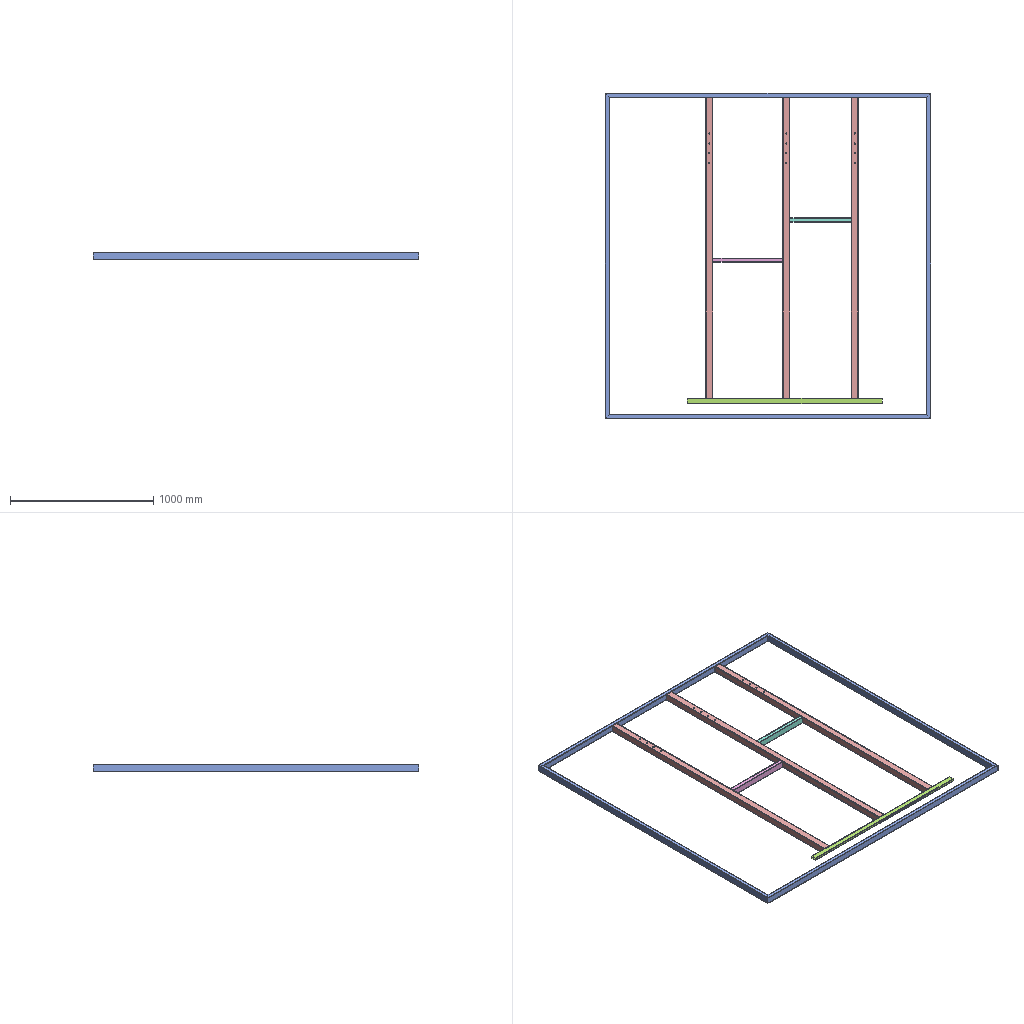Assembly | SolidWorks | 5 different items | 10 placed | box 2270 x 2270 x 50 mm
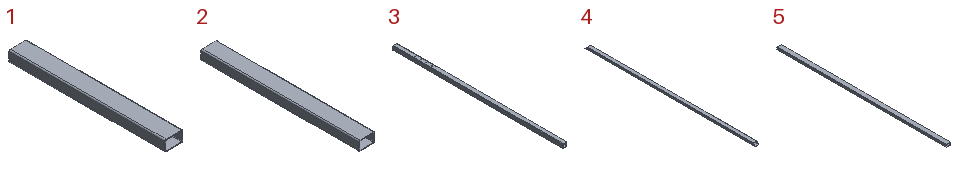Parts list (item | quantity | size | volume | features):
1 | x1 | 50 x 428 x 30 mm | 144560 mm3 | features Extrusion 1
2 | x1 | 50 x 488 x 30 mm | 164826 mm3 | features Extrusion 1
3 | x3 | 50 x 2097 x 50 mm | 900278 mm3 | features Extrusion 1, ICE 1
4 | x4 | 50 x 2270 x 30 mm | 756578 mm3 | features Extrusion 1, ICE 1
5 | x1 | 40 x 1360 x 20 mm | 334231 mm3 | features Extrusion 1
Mates (type | each side: item.copy, entity, surface, feature):
Coincident | 3.1 face plane Boss-Extrude1 | 3.2 face plane Boss-Extrude1 | 2 times
Parallel | 3.2 face plane Boss-Extrude1 | 2.1 face plane Boss-Extrude1
Coincident | 3.2 face plane Boss-Extrude1 | 2.1 face plane Boss-Extrude1 | 2 times
Coincident | 3.1 face plane Boss-Extrude1 | 2.1 face plane Boss-Extrude1
Coincident | 3.1 edge | 4.1 face plane Boss-Extrude1
Coincident | 3.1 face plane Boss-Extrude1 | 4.1 face plane Boss-Extrude1
Coincident | 3.2 face plane Boss-Extrude1 | 4.1 face plane Boss-Extrude1
Coincident | 3.2 face plane Boss-Extrude1 | 4.2 face plane Boss-Extrude1
Coincident | 4.1 face plane Cut-Extrude1 | 4.2 face plane Cut-Extrude1
Coincident | 4.1 face plane Boss-Extrude1 | 4.2 edge
Coincident | 4.3 face plane Boss-Extrude1 | 4.2 face plane Boss-Extrude1
Coincident | 4.3 face plane Cut-Extrude1 | 4.2 face plane Cut-Extrude1
Coincident | 4.3 edge | 4.2 face plane Boss-Extrude1
Coincident | 3.1 face plane Boss-Extrude1 | 1.1 face plane Boss-Extrude1 | 2 times
Coincident | 1.1 face plane Boss-Extrude1 | 3.3 face plane Boss-Extrude1 | 2 times
Coincident | 4.1 face plane Boss-Extrude1 | 3.3 face plane Boss-Extrude1
Coincident | 4.1 face plane Boss-Extrude1 | 4.4 face plane Boss-Extrude1
Coincident | 4.1 face plane Cut-Extrude1 | 4.4 face plane Cut-Extrude1
Coincident | 4.1 edge | 4.4 edge
Coincident | 3.1 face plane Boss-Extrude1 | 5.1 face plane Boss-Extrude1 | 2 times